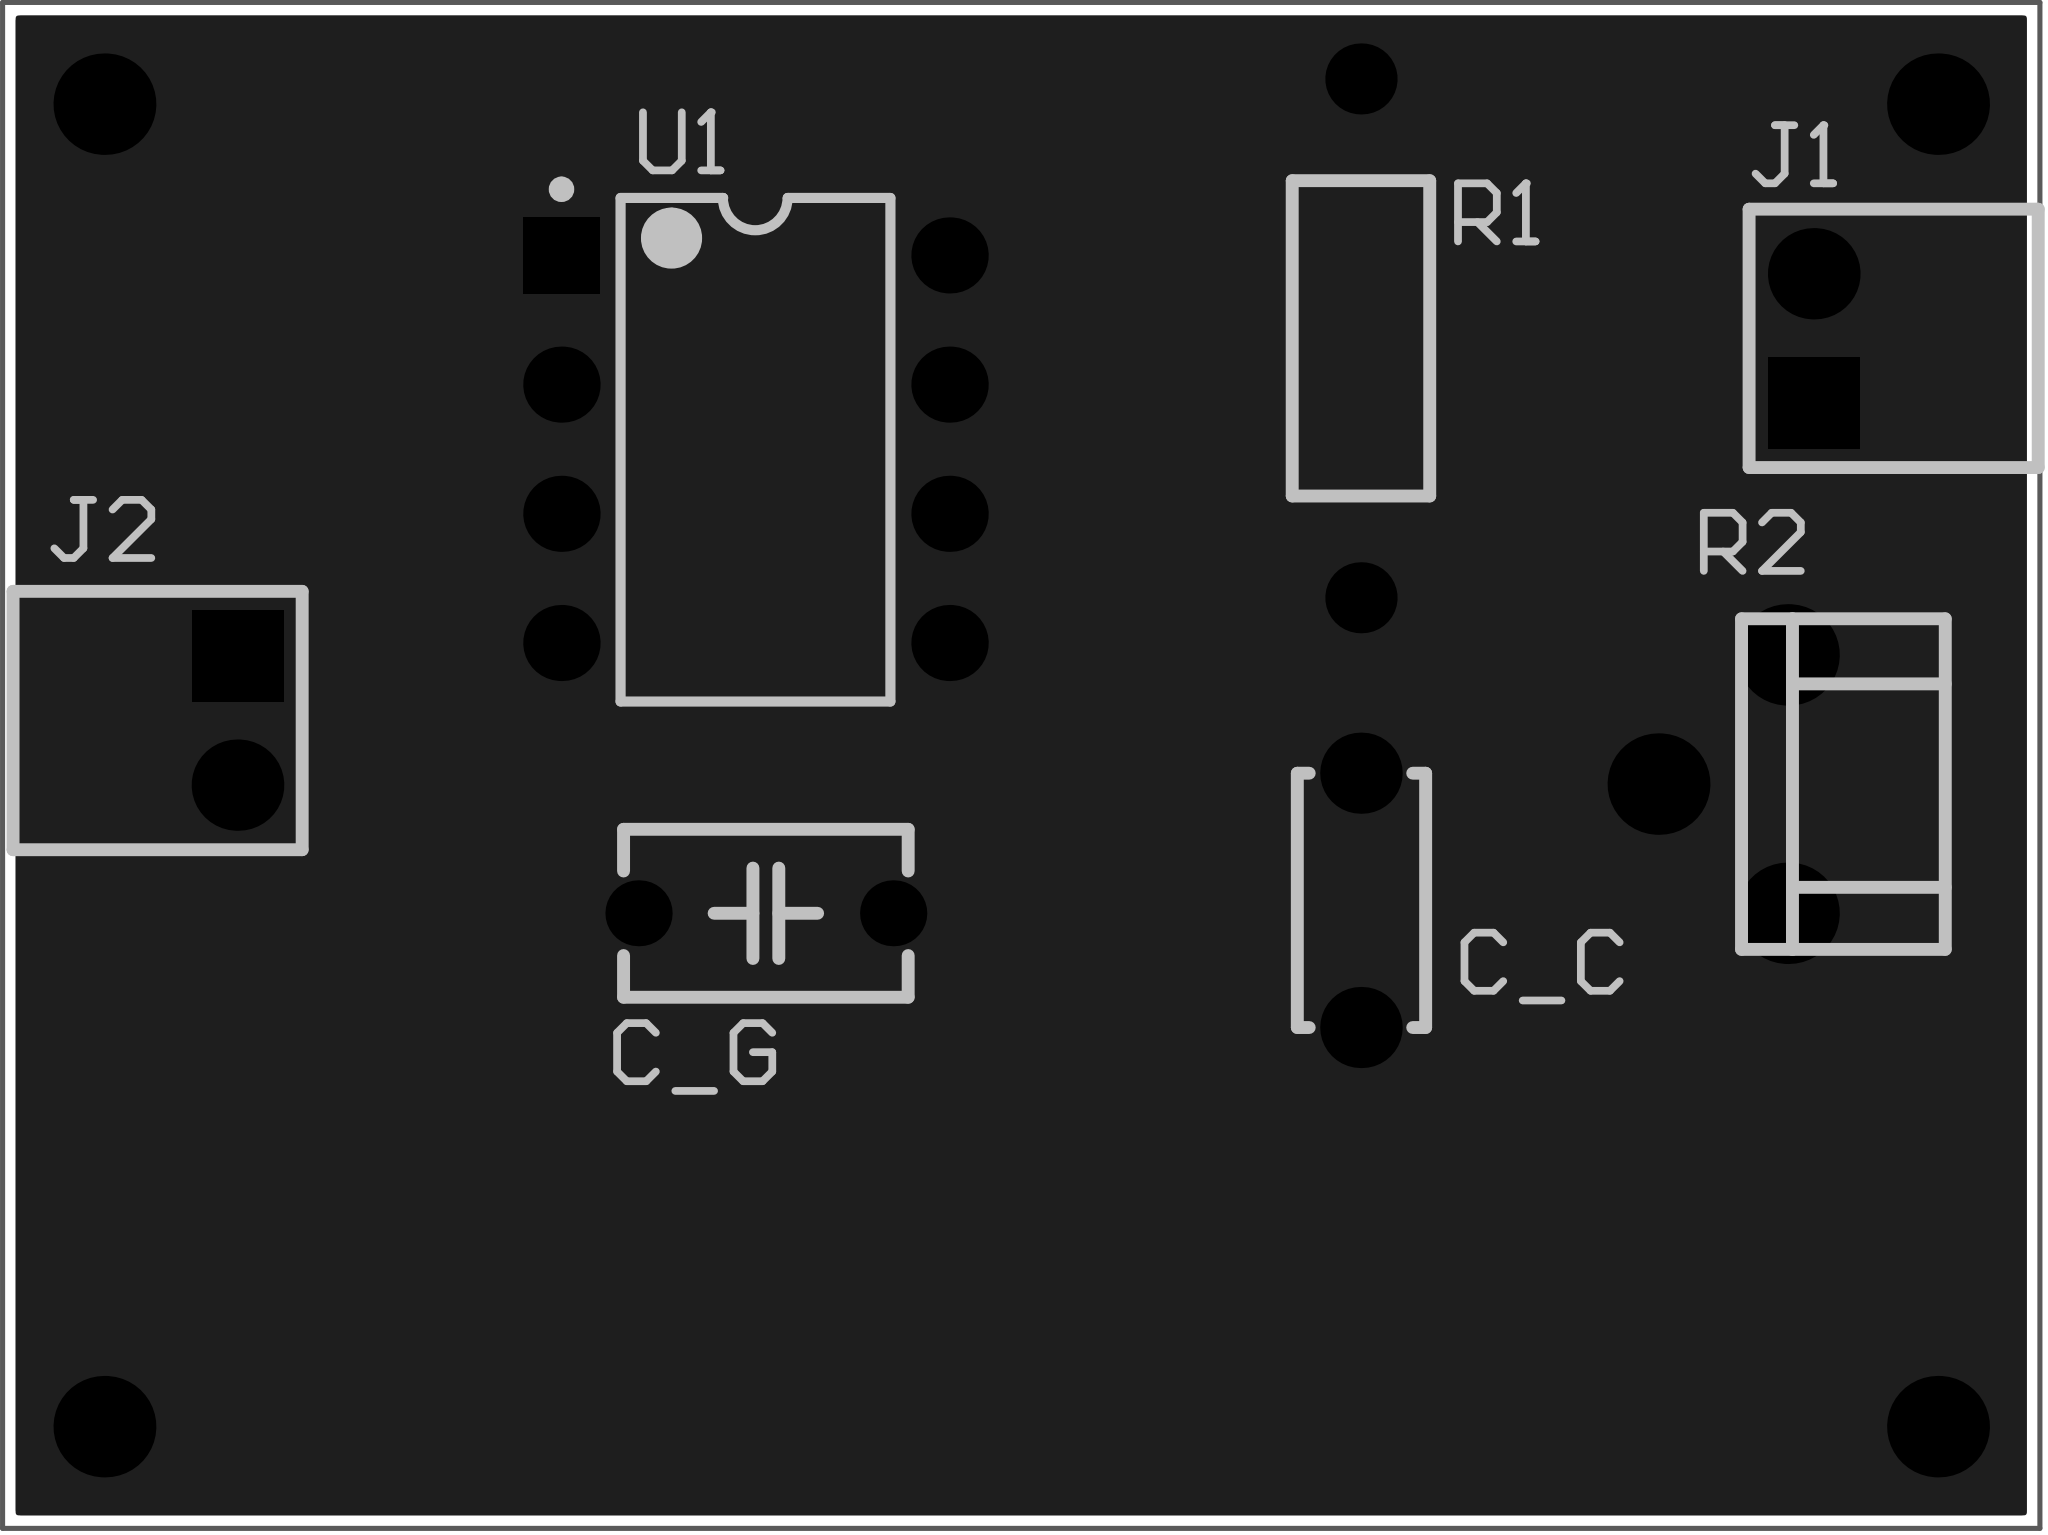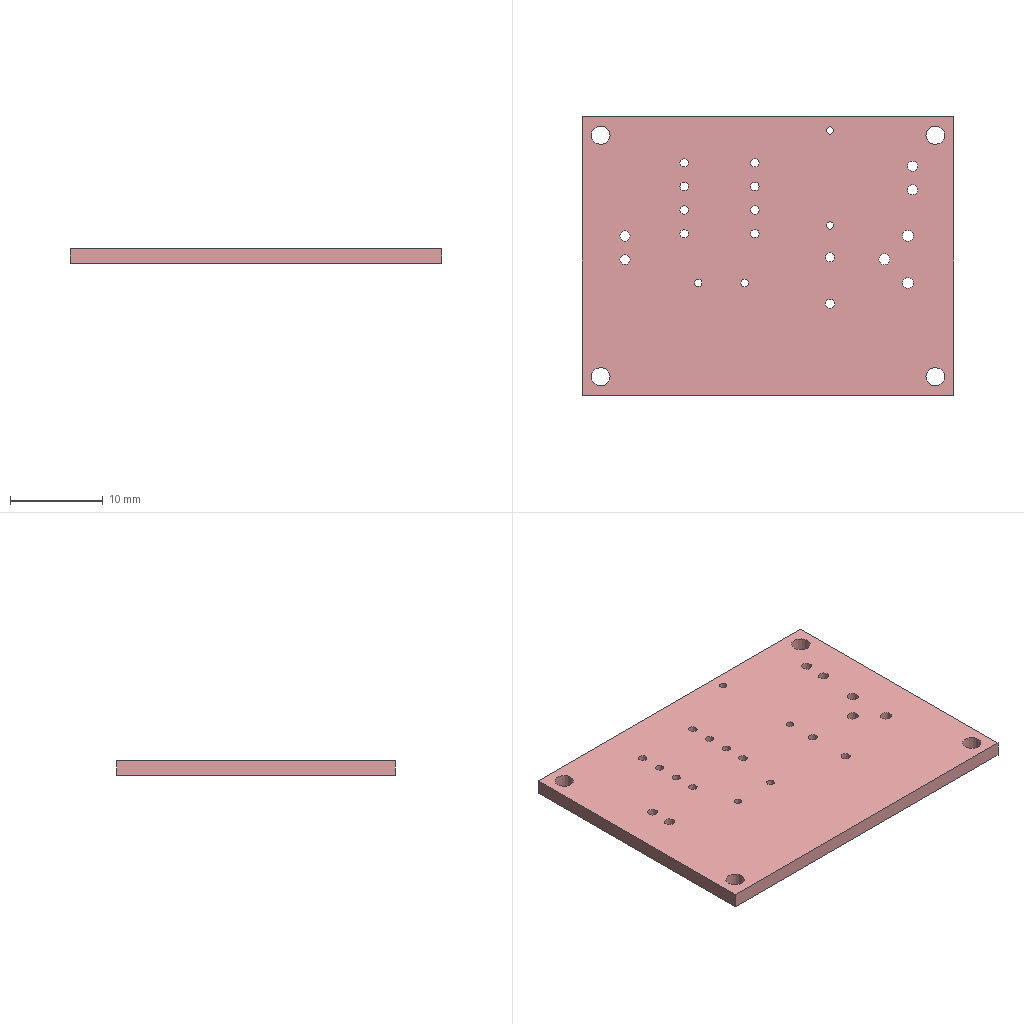Circuit board layout | Altium Designer | box 40 x 30 x 1.6 mm
Layer stack:
# Altium Designer layer stack of  (unit mm; dielectric type: 0 none, 1 core, 2 prepreg, 3 surface material)
index,name,kind,layer,copper_thickness_mm,dielectric_type,dielectric_thickness_mm,dielectric_material,dielectric_constant
0,Top Paste Mask Layer,other,,,,,,
1,Top Silkscreen Layer,other,,,,,,
2,Top Solder Mask Layer,dielectric,,,3,0.01,,3.3
3,Top Layer,copper,Top Layer,0.035,,,,
4,Dielectric1,dielectric,,,3,1.51,FR4,4.5
5,Bottom Layer,copper,Bottom Layer,0.035,,,,
6,Bottom Solder Mask Layer,dielectric,,,3,0.01,,3.3
7,Bottom Silkscreen Layer,other,,,,,,
8,Bottom Paste Mask Layer,other,,,,,,
# drill layer pairs: low layer,high layer
drill_pair,Top Layer,Bottom Layer
Part placement:
Designator,Comment,Layer,Footprint,Center-X(mm),Center-Y(mm),Rotation
J1,,TopLayer,HDR-TH_2P-P2.54-V-M-1,111.76,99.596,90
J2,,TopLayer,HDR-TH_2P-P2.54-V-M-1,80.812,92.082,270
C_C,100nF,TopLayer,CAP-TH_L5.0-W2.5-P5.00-D1.0,102.87,88.547,90
R1,1kΩ,TopLayer,RES-TH_BD2.7-L6.2-P10.20-D0.4,102.87,99.596,90
R2,1MΩ,TopLayer,RES-ADJ-TH_RM063-103,109.982,90.833,90
C_G,10nF,TopLayer,CAP-TH_L5.5-W3.0-P5.00-D0.6,91.186,88.293,0
U1,NE555P,TopLayer,DIP-8_L9.8-W6.6-P2.54-LS7.6-BL,90.982,97.416,270
Pad and via stacks:
# Altium Designer via and pad stacks of  (unit mm). Each distinct definition once, with the count of objects using it.
# via: kind,start_layer,end_layer,hole_mm,diameter_mm,mode(0 simple;1 top-mid-bottom;2 full stack),diameter_per_layer,count,example_net
# pad: kind,layer,hole_mm,hole_type(0 round;1 square;2 slot),plating,top_size,top_shape(1 round;2 rect;3 octagon;9 rounded rect),mid_size,bottom_size,mode,footprint,size_per_layer,count,example
pad,Multi-Layer,1.1,0,plated,1.8x1.8,1,1.8x1.8,1.8x1.8,0,HDR-TH_2P-P2.54-V-M-1,,2,J1.2
pad,Multi-Layer,1.1,0,plated,1.8x1.8,2,1.8x1.8,1.8x1.8,0,HDR-TH_2P-P2.54-V-M-1,,2,J1.1
pad,Multi-Layer,2,0,plated,2x2,1,2x2,2x2,0,,,4,1
pad,Multi-Layer,1,0,plated,1.6x1.6,1,1.6x1.6,1.6x1.6,0,CAP-TH_L5.0-W2.5-P5.00-D1.0,,2,C_C.1
pad,Multi-Layer,0.8,0,plated,1.4x1.4,1,1.4x1.4,1.4x1.4,0,RES-TH_BD2.7-L6.2-P10.20-D0.4,,2,R1.1
pad,Multi-Layer,1.2,0,plated,2x2,1,2x2,2x2,0,RES-ADJ-TH_RM063-103,,3,R2.1
pad,Multi-Layer,0.8,0,plated,1.3x1.3,1,1.3x1.3,1.3x1.3,0,CAP-TH_L5.5-W3.0-P5.00-D0.6,,2,C_G.2
pad,Multi-Layer,0.9,0,plated,1.5x1.5,2,1.5x1.5,1.5x1.5,0,DIP-8_L9.8-W6.6-P2.54-LS7.6-BL,,1,U1.1
pad,Multi-Layer,0.9,0,plated,1.5x1.5,1,1.5x1.5,1.5x1.5,0,DIP-8_L9.8-W6.6-P2.54-LS7.6-BL,,7,U1.2
Copper pours:
name,layer,net,type(0 solid;1 hatched;2 none)
Top Layer-GND,Top Layer,GND,0
Bottom Layer-GND,Bottom Layer,GND,0
Design rules, without the lines most boards share:
# Altium Designer design rules of  (exported by Altium Designer, unit mm)
# columns: name | kind | enabled | priority | scope1 | scope2 | descriptor | typed fields (field=value)
creepage | 65 | enabled | 1 | All | All | Creepage Distance Constraint =(0mil) (All),(All) |